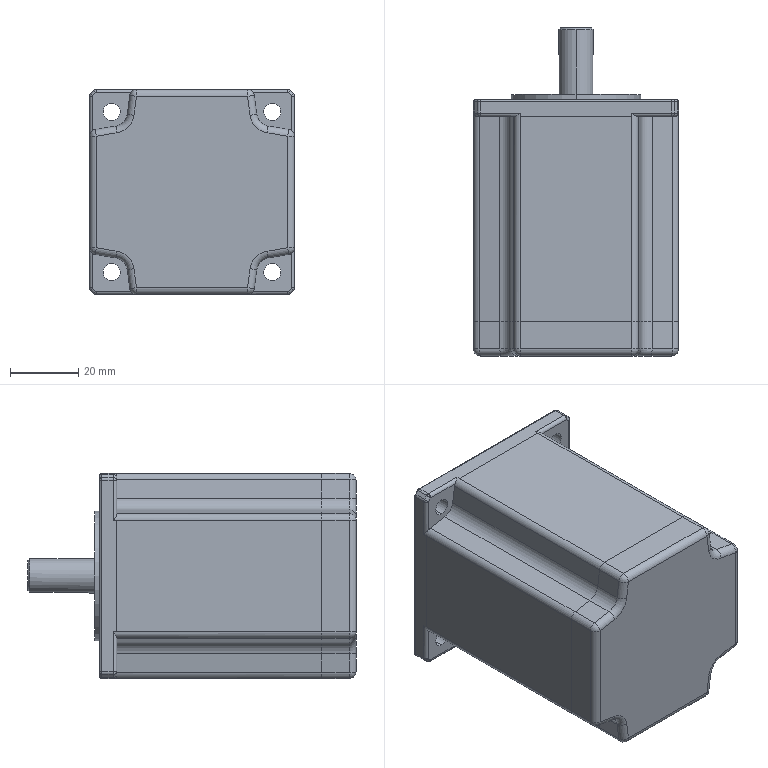Part | STEP file | Stepper motor 24HS8404-10PJ3 | 1 solid | 152 faces | box 60 x 96 x 60 mm | volume 237550 mm3 | cylinder 79 | plane 44 | sphere 16 | torus 12 | cone 1 | commonest cylinder face diameters 4 x28 2 x20 1 x8 5 x8 8 x8 10 x2